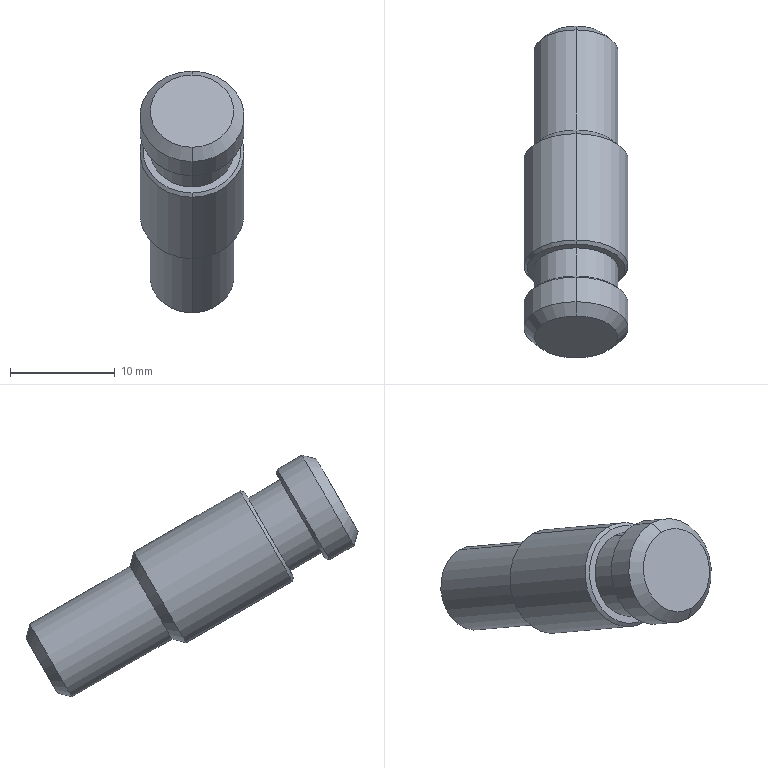Part | SolidWorks | features BaseBody 1 | 1 solid | 22 faces | box 9.95 x 31.633 x 23.023 mm | volume 2058 mm3 | cone 10 | cylinder 8 | plane 4 | commonest cylinder face diameters 8 x4 9.95 x4
STEP:
#1=CARTESIAN_POINT('',(-217.,-182.426,71.656));
#2=VERTEX_POINT('',#1);
#3=CARTESIAN_POINT('',(-217.,-177.451,80.273));
#4=VERTEX_POINT('',#3);
#5=CARTESIAN_POINT('',(-217.,-179.938,75.964));
#6=DIRECTION('',(0.,-0.866,0.5));
#7=DIRECTION('',(0.,-0.5,-0.866));
#8=AXIS2_PLACEMENT_3D('',#5,#6,#7);
#9=CIRCLE('',#8,4.975);
#10=EDGE_CURVE('',#2,#4,#9,.T.);
#11=ORIENTED_EDGE('',*,*,#10,.T.);
#12=CARTESIAN_POINT('',(-217.,-187.583,86.123));
#13=VERTEX_POINT('',#12);
#14=CARTESIAN_POINT('',(-217.,-166.193,73.773));
#15=DIRECTION('',(0.,-0.866,0.5));
#16=VECTOR('',#15,1000.);
#17=LINE('',#14,#16);
#18=EDGE_CURVE('',#4,#13,#17,.T.);
#19=ORIENTED_EDGE('',*,*,#18,.T.);
#20=CARTESIAN_POINT('',(-217.,-192.558,77.506));
#21=VERTEX_POINT('',#20);
#22=CARTESIAN_POINT('',(-217.,-190.071,81.814));
#23=DIRECTION('',(0.,0.866,-0.5));
#24=DIRECTION('',(0.,-0.5,-0.866));
#25=AXIS2_PLACEMENT_3D('',#22,#23,#24);
#26=CIRCLE('',#25,4.975);
#27=EDGE_CURVE('',#13,#21,#26,.T.);
#28=ORIENTED_EDGE('',*,*,#27,.T.);
#29=CARTESIAN_POINT('',(-217.,-171.168,65.156));
#30=DIRECTION('',(0.,-0.866,0.5));
#31=VECTOR('',#30,1000.);
#32=LINE('',#29,#31);
#33=EDGE_CURVE('',#2,#21,#32,.T.);
#34=ORIENTED_EDGE('',*,*,#33,.F.);
#35=EDGE_LOOP('',(#11,#19,#28,#34));
#36=FACE_OUTER_BOUND('',#35,.T.);
#37=CARTESIAN_POINT('',(-217.,-168.68,69.464));
#38=DIRECTION('',(0.,-0.866,0.5));
#39=DIRECTION('',(0.,-0.5,-0.866));
#40=AXIS2_PLACEMENT_3D('',#37,#38,#39);
#41=CYLINDRICAL_SURFACE('',#40,4.975);
#42=ADVANCED_FACE('',(#36),#41,.T.);
#43=CARTESIAN_POINT('',(-217.,-187.993,86.013));
#44=VERTEX_POINT('',#43);
#45=CARTESIAN_POINT('',(-217.,-192.668,77.916));
#46=VERTEX_POINT('',#45);
#47=CARTESIAN_POINT('',(-217.,-190.331,81.964));
#48=DIRECTION('',(0.,0.866,-0.5));
#49=DIRECTION('',(0.,0.5,0.866));
#50=AXIS2_PLACEMENT_3D('',#47,#48,#49);
#51=CIRCLE('',#50,4.675);
#52=EDGE_CURVE('',#44,#46,#51,.T.);
#53=ORIENTED_EDGE('',*,*,#52,.T.);
#54=CARTESIAN_POINT('',(-217.,-192.558,77.506));
#55=DIRECTION('',(0.,0.2588,-0.9659));
#56=VECTOR('',#55,1000.);
#57=LINE('',#54,#56);
#58=EDGE_CURVE('',#46,#21,#57,.T.);
#59=ORIENTED_EDGE('',*,*,#58,.T.);
#60=ORIENTED_EDGE('',*,*,#27,.F.);
#61=CARTESIAN_POINT('',(-217.,-187.583,86.123));
#62=DIRECTION('',(0.,0.9659,0.2588));
#63=VECTOR('',#62,1000.);
#64=LINE('',#61,#63);
#65=EDGE_CURVE('',#44,#13,#64,.T.);
#66=ORIENTED_EDGE('',*,*,#65,.F.);
#67=EDGE_LOOP('',(#53,#59,#60,#66));
#68=FACE_OUTER_BOUND('',#67,.T.);
#69=CARTESIAN_POINT('',(-217.,-190.071,81.814));
#70=DIRECTION('',(0.,0.866,-0.5));
#71=DIRECTION('',(0.,0.5,0.866));
#72=AXIS2_PLACEMENT_3D('',#69,#70,#71);
#73=CONICAL_SURFACE('',#72,4.975,0.7854);
#74=ADVANCED_FACE('',(#68),#73,.T.);
#75=CARTESIAN_POINT('',(-217.,-181.094,72.013));
#76=VERTEX_POINT('',#75);
#77=CARTESIAN_POINT('',(-217.,-177.094,78.941));
#78=VERTEX_POINT('',#77);
#79=CARTESIAN_POINT('',(-217.,-179.094,75.477));
#80=DIRECTION('',(0.,-0.866,0.5));
#81=DIRECTION('',(0.,-0.5,-0.866));
#82=AXIS2_PLACEMENT_3D('',#79,#80,#81);
#83=CIRCLE('',#82,4.);
#84=EDGE_CURVE('',#76,#78,#83,.T.);
#85=ORIENTED_EDGE('',*,*,#84,.T.);
#86=CARTESIAN_POINT('',(-217.,-177.451,80.273));
#87=DIRECTION('',(0.,-0.2588,0.9659));
#88=VECTOR('',#87,1000.);
#89=LINE('',#86,#88);
#90=EDGE_CURVE('',#78,#4,#89,.T.);
#91=ORIENTED_EDGE('',*,*,#90,.T.);
#92=ORIENTED_EDGE('',*,*,#10,.F.);
#93=CARTESIAN_POINT('',(-217.,-182.426,71.656));
#94=DIRECTION('',(0.,-0.9659,-0.2588));
#95=VECTOR('',#94,1000.);
#96=LINE('',#93,#95);
#97=EDGE_CURVE('',#76,#2,#96,.T.);
#98=ORIENTED_EDGE('',*,*,#97,.F.);
#99=EDGE_LOOP('',(#85,#91,#92,#98));
#100=FACE_OUTER_BOUND('',#99,.T.);
#101=CARTESIAN_POINT('',(-217.,-179.938,75.964));
#102=DIRECTION('',(0.,-0.866,0.5));
#103=DIRECTION('',(0.,-0.5,-0.866));
#104=AXIS2_PLACEMENT_3D('',#101,#102,#103);
#105=CONICAL_SURFACE('',#104,4.975,0.7854);
#106=ADVANCED_FACE('',(#100),#105,.T.);
#107=ORIENTED_EDGE('',*,*,#84,.F.);
#108=CARTESIAN_POINT('',(-217.,-171.546,66.5));
#109=VERTEX_POINT('',#108);
#110=CARTESIAN_POINT('',(-217.,-181.072,72.));
#111=DIRECTION('',(0.,0.866,-0.5));
#112=VECTOR('',#111,1000.);
#113=LINE('',#110,#112);
#114=EDGE_CURVE('',#76,#109,#113,.T.);
#115=ORIENTED_EDGE('',*,*,#114,.T.);
#116=CARTESIAN_POINT('',(-217.,-167.546,73.429));
#117=VERTEX_POINT('',#116);
#118=CARTESIAN_POINT('',(-217.,-169.546,69.964));
#119=DIRECTION('',(0.,-0.866,0.5));
#120=DIRECTION('',(0.,0.5,0.866));
#121=AXIS2_PLACEMENT_3D('',#118,#119,#120);
#122=CIRCLE('',#121,4.);
#123=EDGE_CURVE('',#109,#117,#122,.T.);
#124=ORIENTED_EDGE('',*,*,#123,.T.);
#125=CARTESIAN_POINT('',(-217.,-177.072,78.929));
#126=DIRECTION('',(0.,0.866,-0.5));
#127=VECTOR('',#126,1000.);
#128=LINE('',#125,#127);
#129=EDGE_CURVE('',#78,#117,#128,.T.);
#130=ORIENTED_EDGE('',*,*,#129,.F.);
#131=EDGE_LOOP('',(#107,#115,#124,#130));
#132=FACE_OUTER_BOUND('',#131,.T.);
#133=CARTESIAN_POINT('',(-217.,-179.072,75.464));
#134=DIRECTION('',(0.,0.866,-0.5));
#135=DIRECTION('',(0.,0.5,0.866));
#136=AXIS2_PLACEMENT_3D('',#133,#134,#135);
#137=CYLINDRICAL_SURFACE('',#136,4.);
#138=ADVANCED_FACE('',(#132),#137,.T.);
#139=CARTESIAN_POINT('',(-217.,-188.331,85.429));
#140=VERTEX_POINT('',#139);
#141=CARTESIAN_POINT('',(-217.,-192.331,78.5));
#142=VERTEX_POINT('',#141);
#143=CARTESIAN_POINT('',(-217.,-190.331,81.964));
#144=DIRECTION('',(0.,0.866,-0.5));
#145=DIRECTION('',(0.,-0.5,-0.866));
#146=AXIS2_PLACEMENT_3D('',#143,#144,#145);
#147=CIRCLE('',#146,4.);
#148=EDGE_CURVE('',#140,#142,#147,.T.);
#149=ORIENTED_EDGE('',*,*,#148,.F.);
#150=CARTESIAN_POINT('',(-217.,-191.362,87.179));
#151=VERTEX_POINT('',#150);
#152=CARTESIAN_POINT('',(-217.,-188.331,85.429));
#153=DIRECTION('',(0.,-0.866,0.5));
#154=VECTOR('',#153,1000.);
#155=LINE('',#152,#154);
#156=EDGE_CURVE('',#140,#151,#155,.T.);
#157=ORIENTED_EDGE('',*,*,#156,.T.);
#158=CARTESIAN_POINT('',(-217.,-195.362,80.25));
#159=VERTEX_POINT('',#158);
#160=CARTESIAN_POINT('',(-217.,-193.362,83.714));
#161=DIRECTION('',(0.,0.866,-0.5));
#162=DIRECTION('',(0.,-0.5,-0.866));
#163=AXIS2_PLACEMENT_3D('',#160,#161,#162);
#164=CIRCLE('',#163,4.);
#165=EDGE_CURVE('',#151,#159,#164,.T.);
#166=ORIENTED_EDGE('',*,*,#165,.T.);
#167=CARTESIAN_POINT('',(-217.,-192.331,78.5));
#168=DIRECTION('',(0.,-0.866,0.5));
#169=VECTOR('',#168,1000.);
#170=LINE('',#167,#169);
#171=EDGE_CURVE('',#142,#159,#170,.T.);
#172=ORIENTED_EDGE('',*,*,#171,.F.);
#173=EDGE_LOOP('',(#149,#157,#166,#172));
#174=FACE_OUTER_BOUND('',#173,.T.);
#175=CARTESIAN_POINT('',(-217.,-190.331,81.964));
#176=DIRECTION('',(0.,-0.866,0.5));
#177=DIRECTION('',(0.,-0.5,-0.866));
#178=AXIS2_PLACEMENT_3D('',#175,#176,#177);
#179=CYLINDRICAL_SURFACE('',#178,4.);
#180=ADVANCED_FACE('',(#174),#179,.T.);
#181=CARTESIAN_POINT('',(-217.,-170.18,66.866));
#182=VERTEX_POINT('',#181);
#183=CARTESIAN_POINT('',(-217.,-167.18,72.062));
#184=VERTEX_POINT('',#183);
#185=CARTESIAN_POINT('',(-217.,-168.68,69.464));
#186=DIRECTION('',(0.,-0.866,0.5));
#187=DIRECTION('',(0.,-0.5,-0.866));
#188=AXIS2_PLACEMENT_3D('',#185,#186,#187);
#189=CIRCLE('',#188,3.);
#190=EDGE_CURVE('',#182,#184,#189,.T.);
#191=ORIENTED_EDGE('',*,*,#190,.T.);
#192=CARTESIAN_POINT('',(-217.,-167.546,73.429));
#193=DIRECTION('',(0.,-0.2588,0.9659));
#194=VECTOR('',#193,1000.);
#195=LINE('',#192,#194);
#196=EDGE_CURVE('',#184,#117,#195,.T.);
#197=ORIENTED_EDGE('',*,*,#196,.T.);
#198=ORIENTED_EDGE('',*,*,#123,.F.);
#199=CARTESIAN_POINT('',(-217.,-171.546,66.5));
#200=DIRECTION('',(0.,-0.9659,-0.2588));
#201=VECTOR('',#200,1000.);
#202=LINE('',#199,#201);
#203=EDGE_CURVE('',#182,#109,#202,.T.);
#204=ORIENTED_EDGE('',*,*,#203,.F.);
#205=EDGE_LOOP('',(#191,#197,#198,#204));
#206=FACE_OUTER_BOUND('',#205,.T.);
#207=CARTESIAN_POINT('',(-217.,-169.546,69.964));
#208=DIRECTION('',(0.,-0.866,0.5));
#209=DIRECTION('',(0.,-0.5,-0.866));
#210=AXIS2_PLACEMENT_3D('',#207,#208,#209);
#211=CONICAL_SURFACE('',#210,4.,0.7854);
#212=ADVANCED_FACE('',(#206),#211,.T.);
#213=CARTESIAN_POINT('',(-217.,-195.699,79.666));
#214=VERTEX_POINT('',#213);
#215=CARTESIAN_POINT('',(-217.,-191.024,87.763));
#216=VERTEX_POINT('',#215);
#217=CARTESIAN_POINT('',(-217.,-193.362,83.714));
#218=DIRECTION('',(0.,-0.866,0.5));
#219=DIRECTION('',(0.,-0.5,-0.866));
#220=AXIS2_PLACEMENT_3D('',#217,#218,#219);
#221=CIRCLE('',#220,4.675);
#222=EDGE_CURVE('',#214,#216,#221,.T.);
#223=ORIENTED_EDGE('',*,*,#222,.T.);
#224=CARTESIAN_POINT('',(-217.,-191.134,88.173));
#225=VERTEX_POINT('',#224);
#226=CARTESIAN_POINT('',(-217.,-191.134,88.173));
#227=DIRECTION('',(0.,-0.2588,0.9659));
#228=VECTOR('',#227,1000.);
#229=LINE('',#226,#228);
#230=EDGE_CURVE('',#216,#225,#229,.T.);
#231=ORIENTED_EDGE('',*,*,#230,.T.);
#232=CARTESIAN_POINT('',(-217.,-196.109,79.556));
#233=VERTEX_POINT('',#232);
#234=CARTESIAN_POINT('',(-217.,-193.622,83.864));
#235=DIRECTION('',(0.,0.866,-0.5));
#236=DIRECTION('',(0.,-0.5,-0.866));
#237=AXIS2_PLACEMENT_3D('',#234,#235,#236);
#238=CIRCLE('',#237,4.975);
#239=EDGE_CURVE('',#225,#233,#238,.T.);
#240=ORIENTED_EDGE('',*,*,#239,.T.);
#241=CARTESIAN_POINT('',(-217.,-196.109,79.556));
#242=DIRECTION('',(0.,-0.9659,-0.2588));
#243=VECTOR('',#242,1000.);
#244=LINE('',#241,#243);
#245=EDGE_CURVE('',#214,#233,#244,.T.);
#246=ORIENTED_EDGE('',*,*,#245,.F.);
#247=EDGE_LOOP('',(#223,#231,#240,#246));
#248=FACE_OUTER_BOUND('',#247,.T.);
#249=CARTESIAN_POINT('',(-217.,-193.622,83.864));
#250=DIRECTION('',(0.,-0.866,0.5));
#251=DIRECTION('',(0.,-0.5,-0.866));
#252=AXIS2_PLACEMENT_3D('',#249,#250,#251);
#253=CONICAL_SURFACE('',#252,4.975,0.7854);
#254=ADVANCED_FACE('',(#248),#253,.T.);
#255=ORIENTED_EDGE('',*,*,#239,.F.);
#256=CARTESIAN_POINT('',(-217.,-193.472,89.523));
#257=VERTEX_POINT('',#256);
#258=CARTESIAN_POINT('',(-217.,-166.193,73.773));
#259=DIRECTION('',(0.,-0.866,0.5));
#260=VECTOR('',#259,1000.);
#261=LINE('',#258,#260);
#262=EDGE_CURVE('',#225,#257,#261,.T.);
#263=ORIENTED_EDGE('',*,*,#262,.T.);
#264=CARTESIAN_POINT('',(-217.,-198.447,80.906));
#265=VERTEX_POINT('',#264);
#266=CARTESIAN_POINT('',(-217.,-195.96,85.214));
#267=DIRECTION('',(0.,0.866,-0.5));
#268=DIRECTION('',(0.,-0.5,-0.866));
#269=AXIS2_PLACEMENT_3D('',#266,#267,#268);
#270=CIRCLE('',#269,4.975);
#271=EDGE_CURVE('',#257,#265,#270,.T.);
#272=ORIENTED_EDGE('',*,*,#271,.T.);
#273=CARTESIAN_POINT('',(-217.,-171.168,65.156));
#274=DIRECTION('',(0.,-0.866,0.5));
#275=VECTOR('',#274,1000.);
#276=LINE('',#273,#275);
#277=EDGE_CURVE('',#233,#265,#276,.T.);
#278=ORIENTED_EDGE('',*,*,#277,.F.);
#279=EDGE_LOOP('',(#255,#263,#272,#278));
#280=FACE_OUTER_BOUND('',#279,.T.);
#281=CARTESIAN_POINT('',(-217.,-168.68,69.464));
#282=DIRECTION('',(0.,-0.866,0.5));
#283=DIRECTION('',(0.,-0.5,-0.866));
#284=AXIS2_PLACEMENT_3D('',#281,#282,#283);
#285=CYLINDRICAL_SURFACE('',#284,4.975);
#286=ADVANCED_FACE('',(#280),#285,.T.);
#287=CARTESIAN_POINT('',(-217.,-194.838,89.157));
#288=VERTEX_POINT('',#287);
#289=CARTESIAN_POINT('',(-217.,-198.813,82.272));
#290=VERTEX_POINT('',#289);
#291=CARTESIAN_POINT('',(-217.,-196.826,85.714));
#292=DIRECTION('',(0.,0.866,-0.5));
#293=DIRECTION('',(0.,0.5,0.866));
#294=AXIS2_PLACEMENT_3D('',#291,#292,#293);
#295=CIRCLE('',#294,3.975);
#296=EDGE_CURVE('',#288,#290,#295,.T.);
#297=ORIENTED_EDGE('',*,*,#296,.T.);
#298=CARTESIAN_POINT('',(-217.,-198.447,80.906));
#299=DIRECTION('',(0.,0.2588,-0.9659));
#300=VECTOR('',#299,1000.);
#301=LINE('',#298,#300);
#302=EDGE_CURVE('',#290,#265,#301,.T.);
#303=ORIENTED_EDGE('',*,*,#302,.T.);
#304=ORIENTED_EDGE('',*,*,#271,.F.);
#305=CARTESIAN_POINT('',(-217.,-193.472,89.523));
#306=DIRECTION('',(0.,0.9659,0.2588));
#307=VECTOR('',#306,1000.);
#308=LINE('',#305,#307);
#309=EDGE_CURVE('',#288,#257,#308,.T.);
#310=ORIENTED_EDGE('',*,*,#309,.F.);
#311=EDGE_LOOP('',(#297,#303,#304,#310));
#312=FACE_OUTER_BOUND('',#311,.T.);
#313=CARTESIAN_POINT('',(-217.,-195.96,85.214));
#314=DIRECTION('',(0.,0.866,-0.5));
#315=DIRECTION('',(0.,0.5,0.866));
#316=AXIS2_PLACEMENT_3D('',#313,#314,#315);
#317=CONICAL_SURFACE('',#316,4.975,0.7854);
#318=ADVANCED_FACE('',(#312),#317,.T.);
#319=ORIENTED_EDGE('',*,*,#296,.F.);
#320=CARTESIAN_POINT('',(-217.,-196.826,85.714));
#321=DIRECTION('',(0.,0.866,-0.5));
#322=DIRECTION('',(0.,0.5,0.866));
#323=AXIS2_PLACEMENT_3D('',#320,#321,#322);
#324=CIRCLE('',#323,3.975);
#325=EDGE_CURVE('',#290,#288,#324,.T.);
#326=ORIENTED_EDGE('',*,*,#325,.F.);
#327=EDGE_LOOP('',(#319,#326));
#328=FACE_OUTER_BOUND('',#327,.T.);
#329=CARTESIAN_POINT('',(-217.,-196.826,85.714));
#330=DIRECTION('',(0.,0.866,-0.5));
#331=DIRECTION('',(-1.,0.,0.));
#332=AXIS2_PLACEMENT_3D('',#329,#330,#331);
#333=PLANE('',#332);
#334=ADVANCED_FACE('',(#328),#333,.F.);
#335=ORIENTED_EDGE('',*,*,#190,.F.);
#336=CARTESIAN_POINT('',(-217.,-168.68,69.464));
#337=DIRECTION('',(0.,-0.866,0.5));
#338=DIRECTION('',(0.,-0.5,-0.866));
#339=AXIS2_PLACEMENT_3D('',#336,#337,#338);
#340=CIRCLE('',#339,3.);
#341=EDGE_CURVE('',#184,#182,#340,.T.);
#342=ORIENTED_EDGE('',*,*,#341,.F.);
#343=EDGE_LOOP('',(#335,#342));
#344=FACE_OUTER_BOUND('',#343,.T.);
#345=CARTESIAN_POINT('',(-217.,-168.68,69.464));
#346=DIRECTION('',(0.,0.866,-0.5));
#347=DIRECTION('',(-1.,0.,0.));
#348=AXIS2_PLACEMENT_3D('',#345,#346,#347);
#349=PLANE('',#348);
#350=ADVANCED_FACE('',(#344),#349,.T.);
#351=CARTESIAN_POINT('',(-217.,-193.362,83.714));
#352=DIRECTION('',(0.,0.866,-0.5));
#353=DIRECTION('',(0.,-0.5,-0.866));
#354=AXIS2_PLACEMENT_3D('',#351,#352,#353);
#355=CIRCLE('',#354,4.);
#356=EDGE_CURVE('',#159,#151,#355,.T.);
#357=ORIENTED_EDGE('',*,*,#356,.F.);
#358=ORIENTED_EDGE('',*,*,#165,.F.);
#359=EDGE_LOOP('',(#357,#358));
#360=FACE_BOUND('',#359,.T.);
#361=ORIENTED_EDGE('',*,*,#222,.F.);
#362=CARTESIAN_POINT('',(-217.,-193.362,83.714));
#363=DIRECTION('',(0.,-0.866,0.5));
#364=DIRECTION('',(0.,-0.5,-0.866));
#365=AXIS2_PLACEMENT_3D('',#362,#363,#364);
#366=CIRCLE('',#365,4.675);
#367=EDGE_CURVE('',#216,#214,#366,.T.);
#368=ORIENTED_EDGE('',*,*,#367,.F.);
#369=EDGE_LOOP('',(#361,#368));
#370=FACE_OUTER_BOUND('',#369,.T.);
#371=CARTESIAN_POINT('',(-217.,-193.362,83.714));
#372=DIRECTION('',(0.,-0.866,0.5));
#373=DIRECTION('',(-1.,0.,0.));
#374=AXIS2_PLACEMENT_3D('',#371,#372,#373);
#375=PLANE('',#374);
#376=ADVANCED_FACE('',(#360,#370),#375,.F.);
#377=CARTESIAN_POINT('',(-217.,-190.331,81.964));
#378=DIRECTION('',(0.,0.866,-0.5));
#379=DIRECTION('',(0.,-0.5,-0.866));
#380=AXIS2_PLACEMENT_3D('',#377,#378,#379);
#381=CIRCLE('',#380,4.);
#382=EDGE_CURVE('',#142,#140,#381,.T.);
#383=ORIENTED_EDGE('',*,*,#382,.T.);
#384=ORIENTED_EDGE('',*,*,#148,.T.);
#385=EDGE_LOOP('',(#383,#384));
#386=FACE_BOUND('',#385,.T.);
#387=ORIENTED_EDGE('',*,*,#52,.F.);
#388=CARTESIAN_POINT('',(-217.,-190.331,81.964));
#389=DIRECTION('',(0.,0.866,-0.5));
#390=DIRECTION('',(0.,0.5,0.866));
#391=AXIS2_PLACEMENT_3D('',#388,#389,#390);
#392=CIRCLE('',#391,4.675);
#393=EDGE_CURVE('',#46,#44,#392,.T.);
#394=ORIENTED_EDGE('',*,*,#393,.F.);
#395=EDGE_LOOP('',(#387,#394));
#396=FACE_OUTER_BOUND('',#395,.T.);
#397=CARTESIAN_POINT('',(-217.,-190.331,81.964));
#398=DIRECTION('',(0.,-0.866,0.5));
#399=DIRECTION('',(-1.,0.,0.));
#400=AXIS2_PLACEMENT_3D('',#397,#398,#399);
#401=PLANE('',#400);
#402=ADVANCED_FACE('',(#386,#396),#401,.T.);
#403=ORIENTED_EDGE('',*,*,#302,.F.);
#404=ORIENTED_EDGE('',*,*,#325,.T.);
#405=ORIENTED_EDGE('',*,*,#309,.T.);
#406=CARTESIAN_POINT('',(-217.,-195.96,85.214));
#407=DIRECTION('',(0.,0.866,-0.5));
#408=DIRECTION('',(0.,-0.5,-0.866));
#409=AXIS2_PLACEMENT_3D('',#406,#407,#408);
#410=CIRCLE('',#409,4.975);
#411=EDGE_CURVE('',#265,#257,#410,.T.);
#412=ORIENTED_EDGE('',*,*,#411,.F.);
#413=EDGE_LOOP('',(#403,#404,#405,#412));
#414=FACE_OUTER_BOUND('',#413,.T.);
#415=CARTESIAN_POINT('',(-217.,-195.96,85.214));
#416=DIRECTION('',(0.,0.866,-0.5));
#417=DIRECTION('',(0.,0.5,0.866));
#418=AXIS2_PLACEMENT_3D('',#415,#416,#417);
#419=CONICAL_SURFACE('',#418,4.975,0.7854);
#420=ADVANCED_FACE('',(#414),#419,.T.);
#421=ORIENTED_EDGE('',*,*,#262,.F.);
#422=CARTESIAN_POINT('',(-217.,-193.622,83.864));
#423=DIRECTION('',(0.,0.866,-0.5));
#424=DIRECTION('',(0.,-0.5,-0.866));
#425=AXIS2_PLACEMENT_3D('',#422,#423,#424);
#426=CIRCLE('',#425,4.975);
#427=EDGE_CURVE('',#233,#225,#426,.T.);
#428=ORIENTED_EDGE('',*,*,#427,.F.);
#429=ORIENTED_EDGE('',*,*,#277,.T.);
#430=ORIENTED_EDGE('',*,*,#411,.T.);
#431=EDGE_LOOP('',(#421,#428,#429,#430));
#432=FACE_OUTER_BOUND('',#431,.T.);
#433=CARTESIAN_POINT('',(-217.,-168.68,69.464));
#434=DIRECTION('',(0.,-0.866,0.5));
#435=DIRECTION('',(0.,-0.5,-0.866));
#436=AXIS2_PLACEMENT_3D('',#433,#434,#435);
#437=CYLINDRICAL_SURFACE('',#436,4.975);
#438=ADVANCED_FACE('',(#432),#437,.T.);
#439=ORIENTED_EDGE('',*,*,#230,.F.);
#440=ORIENTED_EDGE('',*,*,#367,.T.);
#441=ORIENTED_EDGE('',*,*,#245,.T.);
#442=ORIENTED_EDGE('',*,*,#427,.T.);
#443=EDGE_LOOP('',(#439,#440,#441,#442));
#444=FACE_OUTER_BOUND('',#443,.T.);
#445=CARTESIAN_POINT('',(-217.,-193.622,83.864));
#446=DIRECTION('',(0.,-0.866,0.5));
#447=DIRECTION('',(0.,-0.5,-0.866));
#448=AXIS2_PLACEMENT_3D('',#445,#446,#447);
#449=CONICAL_SURFACE('',#448,4.975,0.7854);
#450=ADVANCED_FACE('',(#444),#449,.T.);
#451=ORIENTED_EDGE('',*,*,#196,.F.);
#452=ORIENTED_EDGE('',*,*,#341,.T.);
#453=ORIENTED_EDGE('',*,*,#203,.T.);
#454=CARTESIAN_POINT('',(-217.,-169.546,69.964));
#455=DIRECTION('',(0.,-0.866,0.5));
#456=DIRECTION('',(0.,0.5,0.866));
#457=AXIS2_PLACEMENT_3D('',#454,#455,#456);
#458=CIRCLE('',#457,4.);
#459=EDGE_CURVE('',#117,#109,#458,.T.);
#460=ORIENTED_EDGE('',*,*,#459,.F.);
#461=EDGE_LOOP('',(#451,#452,#453,#460));
#462=FACE_OUTER_BOUND('',#461,.T.);
#463=CARTESIAN_POINT('',(-217.,-169.546,69.964));
#464=DIRECTION('',(0.,-0.866,0.5));
#465=DIRECTION('',(0.,-0.5,-0.866));
#466=AXIS2_PLACEMENT_3D('',#463,#464,#465);
#467=CONICAL_SURFACE('',#466,4.,0.7854);
#468=ADVANCED_FACE('',(#462),#467,.T.);
#469=ORIENTED_EDGE('',*,*,#156,.F.);
#470=ORIENTED_EDGE('',*,*,#382,.F.);
#471=ORIENTED_EDGE('',*,*,#171,.T.);
#472=ORIENTED_EDGE('',*,*,#356,.T.);
#473=EDGE_LOOP('',(#469,#470,#471,#472));
#474=FACE_OUTER_BOUND('',#473,.T.);
#475=CARTESIAN_POINT('',(-217.,-190.331,81.964));
#476=DIRECTION('',(0.,-0.866,0.5));
#477=DIRECTION('',(0.,-0.5,-0.866));
#478=AXIS2_PLACEMENT_3D('',#475,#476,#477);
#479=CYLINDRICAL_SURFACE('',#478,4.);
#480=ADVANCED_FACE('',(#474),#479,.T.);
#481=ORIENTED_EDGE('',*,*,#114,.F.);
#482=CARTESIAN_POINT('',(-217.,-179.094,75.477));
#483=DIRECTION('',(0.,-0.866,0.5));
#484=DIRECTION('',(0.,-0.5,-0.866));
#485=AXIS2_PLACEMENT_3D('',#482,#483,#484);
#486=CIRCLE('',#485,4.);
#487=EDGE_CURVE('',#78,#76,#486,.T.);
#488=ORIENTED_EDGE('',*,*,#487,.F.);
#489=ORIENTED_EDGE('',*,*,#129,.T.);
#490=ORIENTED_EDGE('',*,*,#459,.T.);
#491=EDGE_LOOP('',(#481,#488,#489,#490));
#492=FACE_OUTER_BOUND('',#491,.T.);
#493=CARTESIAN_POINT('',(-217.,-179.072,75.464));
#494=DIRECTION('',(0.,0.866,-0.5));
#495=DIRECTION('',(0.,0.5,0.866));
#496=AXIS2_PLACEMENT_3D('',#493,#494,#495);
#497=CYLINDRICAL_SURFACE('',#496,4.);
#498=ADVANCED_FACE('',(#492),#497,.T.);
#499=ORIENTED_EDGE('',*,*,#90,.F.);
#500=ORIENTED_EDGE('',*,*,#487,.T.);
#501=ORIENTED_EDGE('',*,*,#97,.T.);
#502=CARTESIAN_POINT('',(-217.,-179.938,75.964));
#503=DIRECTION('',(0.,-0.866,0.5));
#504=DIRECTION('',(0.,-0.5,-0.866));
#505=AXIS2_PLACEMENT_3D('',#502,#503,#504);
#506=CIRCLE('',#505,4.975);
#507=EDGE_CURVE('',#4,#2,#506,.T.);
#508=ORIENTED_EDGE('',*,*,#507,.F.);
#509=EDGE_LOOP('',(#499,#500,#501,#508));
#510=FACE_OUTER_BOUND('',#509,.T.);
#511=CARTESIAN_POINT('',(-217.,-179.938,75.964));
#512=DIRECTION('',(0.,-0.866,0.5));
#513=DIRECTION('',(0.,-0.5,-0.866));
#514=AXIS2_PLACEMENT_3D('',#511,#512,#513);
#515=CONICAL_SURFACE('',#514,4.975,0.7854);
#516=ADVANCED_FACE('',(#510),#515,.T.);
#517=ORIENTED_EDGE('',*,*,#58,.F.);
#518=ORIENTED_EDGE('',*,*,#393,.T.);
#519=ORIENTED_EDGE('',*,*,#65,.T.);
#520=CARTESIAN_POINT('',(-217.,-190.071,81.814));
#521=DIRECTION('',(0.,0.866,-0.5));
#522=DIRECTION('',(0.,-0.5,-0.866));
#523=AXIS2_PLACEMENT_3D('',#520,#521,#522);
#524=CIRCLE('',#523,4.975);
#525=EDGE_CURVE('',#21,#13,#524,.T.);
#526=ORIENTED_EDGE('',*,*,#525,.F.);
#527=EDGE_LOOP('',(#517,#518,#519,#526));
#528=FACE_OUTER_BOUND('',#527,.T.);
#529=CARTESIAN_POINT('',(-217.,-190.071,81.814));
#530=DIRECTION('',(0.,0.866,-0.5));
#531=DIRECTION('',(0.,0.5,0.866));
#532=AXIS2_PLACEMENT_3D('',#529,#530,#531);
#533=CONICAL_SURFACE('',#532,4.975,0.7854);
#534=ADVANCED_FACE('',(#528),#533,.T.);
#535=ORIENTED_EDGE('',*,*,#18,.F.);
#536=ORIENTED_EDGE('',*,*,#507,.T.);
#537=ORIENTED_EDGE('',*,*,#33,.T.);
#538=ORIENTED_EDGE('',*,*,#525,.T.);
#539=EDGE_LOOP('',(#535,#536,#537,#538));
#540=FACE_OUTER_BOUND('',#539,.T.);
#541=CARTESIAN_POINT('',(-217.,-168.68,69.464));
#542=DIRECTION('',(0.,-0.866,0.5));
#543=DIRECTION('',(0.,-0.5,-0.866));
#544=AXIS2_PLACEMENT_3D('',#541,#542,#543);
#545=CYLINDRICAL_SURFACE('',#544,4.975);
#546=ADVANCED_FACE('',(#540),#545,.T.);
#547=CLOSED_SHELL('',(#42,#74,#106,#138,#180,#212,#254,#286,#318,#334,#350,#376,#402,#420,#438,#450,#468,#480,#498,#516,#534,#546));
#548=MANIFOLD_SOLID_BREP('',#547);
#549=CARTESIAN_POINT('',(0.,0.,0.));
#550=DIRECTION('',(0.,0.,1.));
#551=DIRECTION('',(1.,0.,0.));
#552=AXIS2_PLACEMENT_3D('',#549,#550,#551);
#553=(LENGTH_UNIT()NAMED_UNIT(*)SI_UNIT(.MILLI.,.METRE.));
#554=UNCERTAINTY_MEASURE_WITH_UNIT(LENGTH_MEASURE(0.00001),#553,'','');
#555=(NAMED_UNIT(*)PLANE_ANGLE_UNIT()SI_UNIT($,.RADIAN.));
#556=(NAMED_UNIT(*)SI_UNIT($,.STERADIAN.)SOLID_ANGLE_UNIT());
#557=(GEOMETRIC_REPRESENTATION_CONTEXT(3)GLOBAL_UNCERTAINTY_ASSIGNED_CONTEXT((#554))GLOBAL_UNIT_ASSIGNED_CONTEXT((#553,#555,#556))REPRESENTATION_CONTEXT('',''));
#558=ADVANCED_BREP_SHAPE_REPRESENTATION('',(#548,#552),#557);